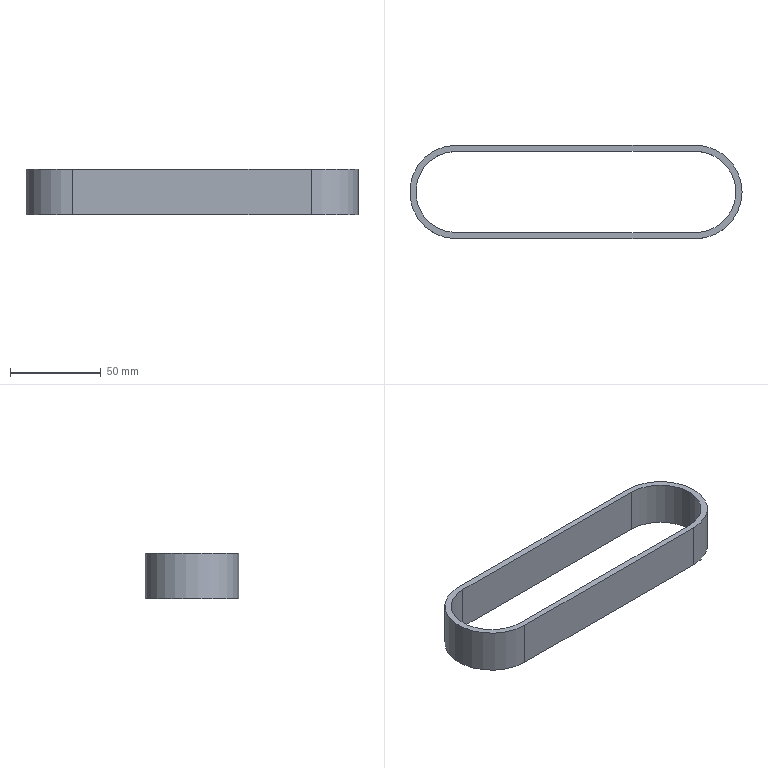Part | STEP file | 1 solid | 12 faces | box 183.34 x 51.65 x 25 mm | volume 35272 mm3 | cylinder 6 | plane 6 | commonest cylinder face diameters 44.85 x3 51.65 x3
STEP:
#1=CARTESIAN_POINT('',(0.,0.,0.));
#2=DIRECTION('',(0.,0.,1.));
#3=DIRECTION('',(1.,0.,0.));
#4=AXIS2_PLACEMENT_3D('',#1,#2,#3);
#5=CARTESIAN_POINT('',(8.226,1.112,-25.));
#6=VERTEX_POINT('',#5);
#7=CARTESIAN_POINT('',(8.226,1.112,0.));
#8=VERTEX_POINT('',#7);
#9=CARTESIAN_POINT('',(8.226,1.112,-25.));
#10=DIRECTION('',(0.,0.,1.));
#11=VECTOR('',#10,1.);
#12=LINE('',#9,#11);
#13=CARTESIAN_POINT('',(8.226,-21.313,-25.));
#14=DIRECTION('',(0.,0.,1.));
#15=DIRECTION('',(1.,0.,0.));
#16=AXIS2_PLACEMENT_3D('',#13,#14,#15);
#17=CYLINDRICAL_SURFACE('',#16,22.425);
#18=CARTESIAN_POINT('',(1.571,0.));
#19=DIRECTION('',(0.,1.));
#20=VECTOR('',#19,1.);
#21=LINE('',#18,#20);
#22=(GEOMETRIC_REPRESENTATION_CONTEXT(2)PARAMETRIC_REPRESENTATION_CONTEXT()REPRESENTATION_CONTEXT('',''));
#23=DEFINITIONAL_REPRESENTATION('',(#21),#22);
#24=PCURVE('',#17,#23);
#25=CARTESIAN_POINT('',(-123.465,1.112,-25.));
#26=DIRECTION('',(0.,-1.,0.));
#27=DIRECTION('',(0.,0.,-1.));
#28=AXIS2_PLACEMENT_3D('',#25,#26,#27);
#29=PLANE('',#28);
#30=CARTESIAN_POINT('',(0.,131.69));
#31=DIRECTION('',(-1.,0.));
#32=VECTOR('',#31,1.);
#33=LINE('',#30,#32);
#34=(GEOMETRIC_REPRESENTATION_CONTEXT(2)PARAMETRIC_REPRESENTATION_CONTEXT()REPRESENTATION_CONTEXT('',''));
#35=DEFINITIONAL_REPRESENTATION('',(#33),#34);
#36=PCURVE('',#29,#35);
#37=SURFACE_CURVE('',#12,(#24,#36),.PCURVE_S1.);
#38=EDGE_CURVE('',#6,#8,#37,.T.);
#39=ORIENTED_EDGE('',*,*,#38,.T.);
#40=CARTESIAN_POINT('',(30.651,-21.313,0.));
#41=VERTEX_POINT('',#40);
#42=CARTESIAN_POINT('',(8.226,-21.313,0.));
#43=DIRECTION('',(0.,0.,-1.));
#44=DIRECTION('',(-1.,0.,0.));
#45=AXIS2_PLACEMENT_3D('',#42,#43,#44);
#46=CIRCLE('',#45,22.425);
#47=CARTESIAN_POINT('',(3.142,25.));
#48=DIRECTION('',(-1.,0.));
#49=VECTOR('',#48,1.);
#50=LINE('',#47,#49);
#51=(GEOMETRIC_REPRESENTATION_CONTEXT(2)PARAMETRIC_REPRESENTATION_CONTEXT()REPRESENTATION_CONTEXT('',''));
#52=DEFINITIONAL_REPRESENTATION('',(#50),#51);
#53=PCURVE('',#17,#52);
#54=CARTESIAN_POINT('',(-123.465,-21.313,0.));
#55=DIRECTION('',(0.,0.,-1.));
#56=DIRECTION('',(-1.,0.,0.));
#57=AXIS2_PLACEMENT_3D('',#54,#55,#56);
#58=PLANE('',#57);
#59=CARTESIAN_POINT('',(-131.69,0.));
#60=DIRECTION('',(1.,0.));
#61=AXIS2_PLACEMENT_2D('',#59,#60);
#62=CIRCLE('',#61,22.425);
#63=(GEOMETRIC_REPRESENTATION_CONTEXT(2)PARAMETRIC_REPRESENTATION_CONTEXT()REPRESENTATION_CONTEXT('',''));
#64=DEFINITIONAL_REPRESENTATION('',(#62),#63);
#65=PCURVE('',#58,#64);
#66=SURFACE_CURVE('',#46,(#53,#65),.PCURVE_S1.);
#67=EDGE_CURVE('',#8,#41,#66,.T.);
#68=ORIENTED_EDGE('',*,*,#67,.T.);
#69=CARTESIAN_POINT('',(30.651,-21.313,-25.));
#70=VERTEX_POINT('',#69);
#71=CARTESIAN_POINT('',(30.651,-21.313,-25.));
#72=DIRECTION('',(0.,0.,1.));
#73=VECTOR('',#72,1.);
#74=LINE('',#71,#73);
#75=CARTESIAN_POINT('',(0.,0.));
#76=DIRECTION('',(0.,1.));
#77=VECTOR('',#76,1.);
#78=LINE('',#75,#77);
#79=(GEOMETRIC_REPRESENTATION_CONTEXT(2)PARAMETRIC_REPRESENTATION_CONTEXT()REPRESENTATION_CONTEXT('',''));
#80=DEFINITIONAL_REPRESENTATION('',(#78),#79);
#81=PCURVE('',#17,#80);
#82=CARTESIAN_POINT('',(8.226,-21.313,-25.));
#83=DIRECTION('',(0.,0.,1.));
#84=DIRECTION('',(1.,0.,0.));
#85=AXIS2_PLACEMENT_3D('',#82,#83,#84);
#86=CYLINDRICAL_SURFACE('',#85,22.425);
#87=CARTESIAN_POINT('',(6.283,0.));
#88=DIRECTION('',(0.,1.));
#89=VECTOR('',#88,1.);
#90=LINE('',#87,#89);
#91=(GEOMETRIC_REPRESENTATION_CONTEXT(2)PARAMETRIC_REPRESENTATION_CONTEXT()REPRESENTATION_CONTEXT('',''));
#92=DEFINITIONAL_REPRESENTATION('',(#90),#91);
#93=PCURVE('',#86,#92);
#94=SURFACE_CURVE('',#74,(#81,#93),.PCURVE_S1.);
#95=EDGE_CURVE('',#70,#41,#94,.T.);
#96=ORIENTED_EDGE('',*,*,#95,.F.);
#97=CARTESIAN_POINT('',(8.226,-21.313,-25.));
#98=DIRECTION('',(0.,0.,-1.));
#99=DIRECTION('',(-1.,0.,0.));
#100=AXIS2_PLACEMENT_3D('',#97,#98,#99);
#101=CIRCLE('',#100,22.425);
#102=CARTESIAN_POINT('',(3.142,0.));
#103=DIRECTION('',(-1.,0.));
#104=VECTOR('',#103,1.);
#105=LINE('',#102,#104);
#106=(GEOMETRIC_REPRESENTATION_CONTEXT(2)PARAMETRIC_REPRESENTATION_CONTEXT()REPRESENTATION_CONTEXT('',''));
#107=DEFINITIONAL_REPRESENTATION('',(#105),#106);
#108=PCURVE('',#17,#107);
#109=CARTESIAN_POINT('',(-123.465,-21.313,-25.));
#110=DIRECTION('',(0.,0.,-1.));
#111=DIRECTION('',(-1.,0.,0.));
#112=AXIS2_PLACEMENT_3D('',#109,#110,#111);
#113=PLANE('',#112);
#114=CARTESIAN_POINT('',(-131.69,0.));
#115=DIRECTION('',(1.,0.));
#116=AXIS2_PLACEMENT_2D('',#114,#115);
#117=CIRCLE('',#116,22.425);
#118=(GEOMETRIC_REPRESENTATION_CONTEXT(2)PARAMETRIC_REPRESENTATION_CONTEXT()REPRESENTATION_CONTEXT('',''));
#119=DEFINITIONAL_REPRESENTATION('',(#117),#118);
#120=PCURVE('',#113,#119);
#121=SURFACE_CURVE('',#101,(#108,#120),.PCURVE_S1.);
#122=EDGE_CURVE('',#6,#70,#121,.T.);
#123=ORIENTED_EDGE('',*,*,#122,.F.);
#124=EDGE_LOOP('',(#39,#68,#96,#123));
#125=FACE_BOUND('',#124,.F.);
#126=ADVANCED_FACE('',(#125),#17,.F.);
#127=CARTESIAN_POINT('',(34.051,-21.313,-25.));
#128=VERTEX_POINT('',#127);
#129=CARTESIAN_POINT('',(8.226,-47.138,-25.));
#130=VERTEX_POINT('',#129);
#131=CARTESIAN_POINT('',(8.226,-21.313,-25.));
#132=DIRECTION('',(0.,0.,-1.));
#133=DIRECTION('',(-1.,0.,0.));
#134=AXIS2_PLACEMENT_3D('',#131,#132,#133);
#135=CIRCLE('',#134,25.825);
#136=CARTESIAN_POINT('',(8.226,-21.313,-25.));
#137=DIRECTION('',(0.,0.,1.));
#138=DIRECTION('',(1.,0.,0.));
#139=AXIS2_PLACEMENT_3D('',#136,#137,#138);
#140=CYLINDRICAL_SURFACE('',#139,25.825);
#141=CARTESIAN_POINT('',(9.425,0.));
#142=DIRECTION('',(-1.,0.));
#143=VECTOR('',#142,1.);
#144=LINE('',#141,#143);
#145=(GEOMETRIC_REPRESENTATION_CONTEXT(2)PARAMETRIC_REPRESENTATION_CONTEXT()REPRESENTATION_CONTEXT('',''));
#146=DEFINITIONAL_REPRESENTATION('',(#144),#145);
#147=PCURVE('',#140,#146);
#148=CARTESIAN_POINT('',(-131.69,0.));
#149=DIRECTION('',(1.,0.));
#150=AXIS2_PLACEMENT_2D('',#148,#149);
#151=CIRCLE('',#150,25.825);
#152=(GEOMETRIC_REPRESENTATION_CONTEXT(2)PARAMETRIC_REPRESENTATION_CONTEXT()REPRESENTATION_CONTEXT('',''));
#153=DEFINITIONAL_REPRESENTATION('',(#151),#152);
#154=PCURVE('',#113,#153);
#155=SURFACE_CURVE('',#135,(#147,#154),.PCURVE_S1.);
#156=EDGE_CURVE('',#128,#130,#155,.T.);
#157=ORIENTED_EDGE('',*,*,#156,.F.);
#158=CARTESIAN_POINT('',(34.051,-21.313,0.));
#159=VERTEX_POINT('',#158);
#160=CARTESIAN_POINT('',(34.051,-21.313,-25.));
#161=DIRECTION('',(0.,0.,1.));
#162=VECTOR('',#161,1.);
#163=LINE('',#160,#162);
#164=CARTESIAN_POINT('',(6.283,0.));
#165=DIRECTION('',(0.,1.));
#166=VECTOR('',#165,1.);
#167=LINE('',#164,#166);
#168=(GEOMETRIC_REPRESENTATION_CONTEXT(2)PARAMETRIC_REPRESENTATION_CONTEXT()REPRESENTATION_CONTEXT('',''));
#169=DEFINITIONAL_REPRESENTATION('',(#167),#168);
#170=PCURVE('',#140,#169);
#171=CARTESIAN_POINT('',(8.226,-21.313,-25.));
#172=DIRECTION('',(0.,0.,1.));
#173=DIRECTION('',(1.,0.,0.));
#174=AXIS2_PLACEMENT_3D('',#171,#172,#173);
#175=CYLINDRICAL_SURFACE('',#174,25.825);
#176=CARTESIAN_POINT('',(0.,0.));
#177=DIRECTION('',(0.,1.));
#178=VECTOR('',#177,1.);
#179=LINE('',#176,#178);
#180=(GEOMETRIC_REPRESENTATION_CONTEXT(2)PARAMETRIC_REPRESENTATION_CONTEXT()REPRESENTATION_CONTEXT('',''));
#181=DEFINITIONAL_REPRESENTATION('',(#179),#180);
#182=PCURVE('',#175,#181);
#183=SURFACE_CURVE('',#163,(#170,#182),.PCURVE_S1.);
#184=EDGE_CURVE('',#128,#159,#183,.T.);
#185=ORIENTED_EDGE('',*,*,#184,.T.);
#186=CARTESIAN_POINT('',(8.226,-47.138,0.));
#187=VERTEX_POINT('',#186);
#188=CARTESIAN_POINT('',(8.226,-21.313,0.));
#189=DIRECTION('',(0.,0.,-1.));
#190=DIRECTION('',(-1.,0.,0.));
#191=AXIS2_PLACEMENT_3D('',#188,#189,#190);
#192=CIRCLE('',#191,25.825);
#193=CARTESIAN_POINT('',(9.425,25.));
#194=DIRECTION('',(-1.,0.));
#195=VECTOR('',#194,1.);
#196=LINE('',#193,#195);
#197=(GEOMETRIC_REPRESENTATION_CONTEXT(2)PARAMETRIC_REPRESENTATION_CONTEXT()REPRESENTATION_CONTEXT('',''));
#198=DEFINITIONAL_REPRESENTATION('',(#196),#197);
#199=PCURVE('',#140,#198);
#200=CARTESIAN_POINT('',(-131.69,0.));
#201=DIRECTION('',(1.,0.));
#202=AXIS2_PLACEMENT_2D('',#200,#201);
#203=CIRCLE('',#202,25.825);
#204=(GEOMETRIC_REPRESENTATION_CONTEXT(2)PARAMETRIC_REPRESENTATION_CONTEXT()REPRESENTATION_CONTEXT('',''));
#205=DEFINITIONAL_REPRESENTATION('',(#203),#204);
#206=PCURVE('',#58,#205);
#207=SURFACE_CURVE('',#192,(#199,#206),.PCURVE_S1.);
#208=EDGE_CURVE('',#159,#187,#207,.T.);
#209=ORIENTED_EDGE('',*,*,#208,.T.);
#210=CARTESIAN_POINT('',(8.226,-47.138,-25.));
#211=DIRECTION('',(0.,0.,1.));
#212=VECTOR('',#211,1.);
#213=LINE('',#210,#212);
#214=CARTESIAN_POINT('',(4.712,0.));
#215=DIRECTION('',(0.,1.));
#216=VECTOR('',#215,1.);
#217=LINE('',#214,#216);
#218=(GEOMETRIC_REPRESENTATION_CONTEXT(2)PARAMETRIC_REPRESENTATION_CONTEXT()REPRESENTATION_CONTEXT('',''));
#219=DEFINITIONAL_REPRESENTATION('',(#217),#218);
#220=PCURVE('',#140,#219);
#221=CARTESIAN_POINT('',(-123.465,-47.138,-25.));
#222=DIRECTION('',(0.,1.,0.));
#223=DIRECTION('',(0.,0.,1.));
#224=AXIS2_PLACEMENT_3D('',#221,#222,#223);
#225=PLANE('',#224);
#226=CARTESIAN_POINT('',(0.,131.69));
#227=DIRECTION('',(1.,0.));
#228=VECTOR('',#227,1.);
#229=LINE('',#226,#228);
#230=(GEOMETRIC_REPRESENTATION_CONTEXT(2)PARAMETRIC_REPRESENTATION_CONTEXT()REPRESENTATION_CONTEXT('',''));
#231=DEFINITIONAL_REPRESENTATION('',(#229),#230);
#232=PCURVE('',#225,#231);
#233=SURFACE_CURVE('',#213,(#220,#232),.PCURVE_S1.);
#234=EDGE_CURVE('',#130,#187,#233,.T.);
#235=ORIENTED_EDGE('',*,*,#234,.F.);
#236=EDGE_LOOP('',(#157,#185,#209,#235));
#237=FACE_BOUND('',#236,.T.);
#238=ADVANCED_FACE('',(#237),#140,.T.);
#239=CARTESIAN_POINT('',(-123.465,-47.138,-25.));
#240=VERTEX_POINT('',#239);
#241=CARTESIAN_POINT('',(-123.465,4.512,-25.));
#242=VERTEX_POINT('',#241);
#243=CARTESIAN_POINT('',(-123.465,-21.313,-25.));
#244=DIRECTION('',(0.,0.,-1.));
#245=DIRECTION('',(-1.,0.,0.));
#246=AXIS2_PLACEMENT_3D('',#243,#244,#245);
#247=CIRCLE('',#246,25.825);
#248=CARTESIAN_POINT('',(0.,0.));
#249=DIRECTION('',(1.,0.));
#250=AXIS2_PLACEMENT_2D('',#248,#249);
#251=CIRCLE('',#250,25.825);
#252=(GEOMETRIC_REPRESENTATION_CONTEXT(2)PARAMETRIC_REPRESENTATION_CONTEXT()REPRESENTATION_CONTEXT('',''));
#253=DEFINITIONAL_REPRESENTATION('',(#251),#252);
#254=PCURVE('',#113,#253);
#255=CARTESIAN_POINT('',(-123.465,-21.313,-25.));
#256=DIRECTION('',(0.,0.,1.));
#257=DIRECTION('',(1.,0.,0.));
#258=AXIS2_PLACEMENT_3D('',#255,#256,#257);
#259=CYLINDRICAL_SURFACE('',#258,25.825);
#260=CARTESIAN_POINT('',(9.425,0.));
#261=DIRECTION('',(-1.,0.));
#262=VECTOR('',#261,1.);
#263=LINE('',#260,#262);
#264=(GEOMETRIC_REPRESENTATION_CONTEXT(2)PARAMETRIC_REPRESENTATION_CONTEXT()REPRESENTATION_CONTEXT('',''));
#265=DEFINITIONAL_REPRESENTATION('',(#263),#264);
#266=PCURVE('',#259,#265);
#267=SURFACE_CURVE('',#247,(#254,#266),.PCURVE_S1.);
#268=EDGE_CURVE('',#240,#242,#267,.T.);
#269=ORIENTED_EDGE('',*,*,#268,.T.);
#270=CARTESIAN_POINT('',(8.226,4.512,-25.));
#271=VERTEX_POINT('',#270);
#272=CARTESIAN_POINT('',(-123.465,4.512,-25.));
#273=DIRECTION('',(1.,0.,0.));
#274=VECTOR('',#273,1.);
#275=LINE('',#272,#274);
#276=CARTESIAN_POINT('',(0.,25.825));
#277=DIRECTION('',(-1.,0.));
#278=VECTOR('',#277,1.);
#279=LINE('',#276,#278);
#280=(GEOMETRIC_REPRESENTATION_CONTEXT(2)PARAMETRIC_REPRESENTATION_CONTEXT()REPRESENTATION_CONTEXT('',''));
#281=DEFINITIONAL_REPRESENTATION('',(#279),#280);
#282=PCURVE('',#113,#281);
#283=CARTESIAN_POINT('',(-123.465,4.512,-25.));
#284=DIRECTION('',(0.,-1.,0.));
#285=DIRECTION('',(0.,0.,-1.));
#286=AXIS2_PLACEMENT_3D('',#283,#284,#285);
#287=PLANE('',#286);
#288=CARTESIAN_POINT('',(0.,0.));
#289=DIRECTION('',(0.,1.));
#290=VECTOR('',#289,1.);
#291=LINE('',#288,#290);
#292=(GEOMETRIC_REPRESENTATION_CONTEXT(2)PARAMETRIC_REPRESENTATION_CONTEXT()REPRESENTATION_CONTEXT('',''));
#293=DEFINITIONAL_REPRESENTATION('',(#291),#292);
#294=PCURVE('',#287,#293);
#295=SURFACE_CURVE('',#275,(#282,#294),.PCURVE_S1.);
#296=EDGE_CURVE('',#242,#271,#295,.T.);
#297=ORIENTED_EDGE('',*,*,#296,.T.);
#298=CARTESIAN_POINT('',(8.226,-21.313,-25.));
#299=DIRECTION('',(0.,0.,-1.));
#300=DIRECTION('',(-1.,0.,0.));
#301=AXIS2_PLACEMENT_3D('',#298,#299,#300);
#302=CIRCLE('',#301,25.825);
#303=CARTESIAN_POINT('',(-131.69,0.));
#304=DIRECTION('',(1.,0.));
#305=AXIS2_PLACEMENT_2D('',#303,#304);
#306=CIRCLE('',#305,25.825);
#307=(GEOMETRIC_REPRESENTATION_CONTEXT(2)PARAMETRIC_REPRESENTATION_CONTEXT()REPRESENTATION_CONTEXT('',''));
#308=DEFINITIONAL_REPRESENTATION('',(#306),#307);
#309=PCURVE('',#113,#308);
#310=CARTESIAN_POINT('',(3.142,0.));
#311=DIRECTION('',(-1.,0.));
#312=VECTOR('',#311,1.);
#313=LINE('',#310,#312);
#314=(GEOMETRIC_REPRESENTATION_CONTEXT(2)PARAMETRIC_REPRESENTATION_CONTEXT()REPRESENTATION_CONTEXT('',''));
#315=DEFINITIONAL_REPRESENTATION('',(#313),#314);
#316=PCURVE('',#175,#315);
#317=SURFACE_CURVE('',#302,(#309,#316),.PCURVE_S1.);
#318=EDGE_CURVE('',#271,#128,#317,.T.);
#319=ORIENTED_EDGE('',*,*,#318,.T.);
#320=ORIENTED_EDGE('',*,*,#156,.T.);
#321=CARTESIAN_POINT('',(-123.465,-47.138,-25.));
#322=DIRECTION('',(-1.,0.,0.));
#323=VECTOR('',#322,1.);
#324=LINE('',#321,#323);
#325=CARTESIAN_POINT('',(0.,-25.825));
#326=DIRECTION('',(1.,0.));
#327=VECTOR('',#326,1.);
#328=LINE('',#325,#327);
#329=(GEOMETRIC_REPRESENTATION_CONTEXT(2)PARAMETRIC_REPRESENTATION_CONTEXT()REPRESENTATION_CONTEXT('',''));
#330=DEFINITIONAL_REPRESENTATION('',(#328),#329);
#331=PCURVE('',#113,#330);
#332=CARTESIAN_POINT('',(0.,0.));
#333=DIRECTION('',(0.,-1.));
#334=VECTOR('',#333,1.);
#335=LINE('',#332,#334);
#336=(GEOMETRIC_REPRESENTATION_CONTEXT(2)PARAMETRIC_REPRESENTATION_CONTEXT()REPRESENTATION_CONTEXT('',''));
#337=DEFINITIONAL_REPRESENTATION('',(#335),#336);
#338=PCURVE('',#225,#337);
#339=SURFACE_CURVE('',#324,(#331,#338),.PCURVE_S1.);
#340=EDGE_CURVE('',#130,#240,#339,.T.);
#341=ORIENTED_EDGE('',*,*,#340,.T.);
#342=EDGE_LOOP('',(#269,#297,#319,#320,#341));
#343=FACE_BOUND('',#342,.T.);
#344=CARTESIAN_POINT('',(-123.465,1.112,-25.));
#345=VERTEX_POINT('',#344);
#346=CARTESIAN_POINT('',(-123.465,1.112,-25.));
#347=DIRECTION('',(1.,0.,0.));
#348=VECTOR('',#347,1.);
#349=LINE('',#346,#348);
#350=CARTESIAN_POINT('',(0.,22.425));
#351=DIRECTION('',(-1.,0.));
#352=VECTOR('',#351,1.);
#353=LINE('',#350,#352);
#354=(GEOMETRIC_REPRESENTATION_CONTEXT(2)PARAMETRIC_REPRESENTATION_CONTEXT()REPRESENTATION_CONTEXT('',''));
#355=DEFINITIONAL_REPRESENTATION('',(#353),#354);
#356=PCURVE('',#113,#355);
#357=CARTESIAN_POINT('',(0.,0.));
#358=DIRECTION('',(0.,1.));
#359=VECTOR('',#358,1.);
#360=LINE('',#357,#359);
#361=(GEOMETRIC_REPRESENTATION_CONTEXT(2)PARAMETRIC_REPRESENTATION_CONTEXT()REPRESENTATION_CONTEXT('',''));
#362=DEFINITIONAL_REPRESENTATION('',(#360),#361);
#363=PCURVE('',#29,#362);
#364=SURFACE_CURVE('',#349,(#356,#363),.PCURVE_S1.);
#365=EDGE_CURVE('',#345,#6,#364,.T.);
#366=ORIENTED_EDGE('',*,*,#365,.F.);
#367=CARTESIAN_POINT('',(-123.465,-43.738,-25.));
#368=VERTEX_POINT('',#367);
#369=CARTESIAN_POINT('',(-123.465,-21.313,-25.));
#370=DIRECTION('',(0.,0.,-1.));
#371=DIRECTION('',(-1.,0.,0.));
#372=AXIS2_PLACEMENT_3D('',#369,#370,#371);
#373=CIRCLE('',#372,22.425);
#374=CARTESIAN_POINT('',(0.,0.));
#375=DIRECTION('',(1.,0.));
#376=AXIS2_PLACEMENT_2D('',#374,#375);
#377=CIRCLE('',#376,22.425);
#378=(GEOMETRIC_REPRESENTATION_CONTEXT(2)PARAMETRIC_REPRESENTATION_CONTEXT()REPRESENTATION_CONTEXT('',''));
#379=DEFINITIONAL_REPRESENTATION('',(#377),#378);
#380=PCURVE('',#113,#379);
#381=CARTESIAN_POINT('',(-123.465,-21.313,-25.));
#382=DIRECTION('',(0.,0.,1.));
#383=DIRECTION('',(1.,0.,0.));
#384=AXIS2_PLACEMENT_3D('',#381,#382,#383);
#385=CYLINDRICAL_SURFACE('',#384,22.425);
#386=CARTESIAN_POINT('',(9.425,0.));
#387=DIRECTION('',(-1.,0.));
#388=VECTOR('',#387,1.);
#389=LINE('',#386,#388);
#390=(GEOMETRIC_REPRESENTATION_CONTEXT(2)PARAMETRIC_REPRESENTATION_CONTEXT()REPRESENTATION_CONTEXT('',''));
#391=DEFINITIONAL_REPRESENTATION('',(#389),#390);
#392=PCURVE('',#385,#391);
#393=SURFACE_CURVE('',#373,(#380,#392),.PCURVE_S1.);
#394=EDGE_CURVE('',#368,#345,#393,.T.);
#395=ORIENTED_EDGE('',*,*,#394,.F.);
#396=CARTESIAN_POINT('',(8.226,-43.738,-25.));
#397=VERTEX_POINT('',#396);
#398=CARTESIAN_POINT('',(-123.465,-43.738,-25.));
#399=DIRECTION('',(-1.,0.,0.));
#400=VECTOR('',#399,1.);
#401=LINE('',#398,#400);
#402=CARTESIAN_POINT('',(0.,-22.425));
#403=DIRECTION('',(1.,0.));
#404=VECTOR('',#403,1.);
#405=LINE('',#402,#404);
#406=(GEOMETRIC_REPRESENTATION_CONTEXT(2)PARAMETRIC_REPRESENTATION_CONTEXT()REPRESENTATION_CONTEXT('',''));
#407=DEFINITIONAL_REPRESENTATION('',(#405),#406);
#408=PCURVE('',#113,#407);
#409=CARTESIAN_POINT('',(-123.465,-43.738,-25.));
#410=DIRECTION('',(0.,1.,0.));
#411=DIRECTION('',(0.,0.,1.));
#412=AXIS2_PLACEMENT_3D('',#409,#410,#411);
#413=PLANE('',#412);
#414=CARTESIAN_POINT('',(0.,0.));
#415=DIRECTION('',(0.,-1.));
#416=VECTOR('',#415,1.);
#417=LINE('',#414,#416);
#418=(GEOMETRIC_REPRESENTATION_CONTEXT(2)PARAMETRIC_REPRESENTATION_CONTEXT()REPRESENTATION_CONTEXT('',''));
#419=DEFINITIONAL_REPRESENTATION('',(#417),#418);
#420=PCURVE('',#413,#419);
#421=SURFACE_CURVE('',#401,(#408,#420),.PCURVE_S1.);
#422=EDGE_CURVE('',#397,#368,#421,.T.);
#423=ORIENTED_EDGE('',*,*,#422,.F.);
#424=CARTESIAN_POINT('',(8.226,-21.313,-25.));
#425=DIRECTION('',(0.,0.,-1.));
#426=DIRECTION('',(-1.,0.,0.));
#427=AXIS2_PLACEMENT_3D('',#424,#425,#426);
#428=CIRCLE('',#427,22.425);
#429=CARTESIAN_POINT('',(-131.69,0.));
#430=DIRECTION('',(1.,0.));
#431=AXIS2_PLACEMENT_2D('',#429,#430);
#432=CIRCLE('',#431,22.425);
#433=(GEOMETRIC_REPRESENTATION_CONTEXT(2)PARAMETRIC_REPRESENTATION_CONTEXT()REPRESENTATION_CONTEXT('',''));
#434=DEFINITIONAL_REPRESENTATION('',(#432),#433);
#435=PCURVE('',#113,#434);
#436=CARTESIAN_POINT('',(9.425,0.));
#437=DIRECTION('',(-1.,0.));
#438=VECTOR('',#437,1.);
#439=LINE('',#436,#438);
#440=(GEOMETRIC_REPRESENTATION_CONTEXT(2)PARAMETRIC_REPRESENTATION_CONTEXT()REPRESENTATION_CONTEXT('',''));
#441=DEFINITIONAL_REPRESENTATION('',(#439),#440);
#442=PCURVE('',#86,#441);
#443=SURFACE_CURVE('',#428,(#435,#442),.PCURVE_S1.);
#444=EDGE_CURVE('',#70,#397,#443,.T.);
#445=ORIENTED_EDGE('',*,*,#444,.F.);
#446=ORIENTED_EDGE('',*,*,#122,.F.);
#447=EDGE_LOOP('',(#366,#395,#423,#445,#446));
#448=FACE_BOUND('',#447,.T.);
#449=ADVANCED_FACE('',(#343,#448),#113,.T.);
#450=CARTESIAN_POINT('',(-123.465,-47.138,0.));
#451=VERTEX_POINT('',#450);
#452=CARTESIAN_POINT('',(-123.465,4.512,0.));
#453=VERTEX_POINT('',#452);
#454=CARTESIAN_POINT('',(-123.465,-21.313,0.));
#455=DIRECTION('',(0.,0.,-1.));
#456=DIRECTION('',(-1.,0.,0.));
#457=AXIS2_PLACEMENT_3D('',#454,#455,#456);
#458=CIRCLE('',#457,25.825);
#459=CARTESIAN_POINT('',(0.,0.));
#460=DIRECTION('',(1.,0.));
#461=AXIS2_PLACEMENT_2D('',#459,#460);
#462=CIRCLE('',#461,25.825);
#463=(GEOMETRIC_REPRESENTATION_CONTEXT(2)PARAMETRIC_REPRESENTATION_CONTEXT()REPRESENTATION_CONTEXT('',''));
#464=DEFINITIONAL_REPRESENTATION('',(#462),#463);
#465=PCURVE('',#58,#464);
#466=CARTESIAN_POINT('',(9.425,25.));
#467=DIRECTION('',(-1.,0.));
#468=VECTOR('',#467,1.);
#469=LINE('',#466,#468);
#470=(GEOMETRIC_REPRESENTATION_CONTEXT(2)PARAMETRIC_REPRESENTATION_CONTEXT()REPRESENTATION_CONTEXT('',''));
#471=DEFINITIONAL_REPRESENTATION('',(#469),#470);
#472=PCURVE('',#259,#471);
#473=SURFACE_CURVE('',#458,(#465,#472),.PCURVE_S1.);
#474=EDGE_CURVE('',#451,#453,#473,.T.);
#475=ORIENTED_EDGE('',*,*,#474,.F.);
#476=CARTESIAN_POINT('',(-123.465,-47.138,0.));
#477=DIRECTION('',(-1.,0.,0.));
#478=VECTOR('',#477,1.);
#479=LINE('',#476,#478);
#480=CARTESIAN_POINT('',(0.,-25.825));
#481=DIRECTION('',(1.,0.));
#482=VECTOR('',#481,1.);
#483=LINE('',#480,#482);
#484=(GEOMETRIC_REPRESENTATION_CONTEXT(2)PARAMETRIC_REPRESENTATION_CONTEXT()REPRESENTATION_CONTEXT('',''));
#485=DEFINITIONAL_REPRESENTATION('',(#483),#484);
#486=PCURVE('',#58,#485);
#487=CARTESIAN_POINT('',(25.,0.));
#488=DIRECTION('',(0.,-1.));
#489=VECTOR('',#488,1.);
#490=LINE('',#487,#489);
#491=(GEOMETRIC_REPRESENTATION_CONTEXT(2)PARAMETRIC_REPRESENTATION_CONTEXT()REPRESENTATION_CONTEXT('',''));
#492=DEFINITIONAL_REPRESENTATION('',(#490),#491);
#493=PCURVE('',#225,#492);
#494=SURFACE_CURVE('',#479,(#486,#493),.PCURVE_S1.);
#495=EDGE_CURVE('',#187,#451,#494,.T.);
#496=ORIENTED_EDGE('',*,*,#495,.F.);
#497=ORIENTED_EDGE('',*,*,#208,.F.);
#498=CARTESIAN_POINT('',(8.226,4.512,0.));
#499=VERTEX_POINT('',#498);
#500=CARTESIAN_POINT('',(8.226,-21.313,0.));
#501=DIRECTION('',(0.,0.,-1.));
#502=DIRECTION('',(-1.,0.,0.));
#503=AXIS2_PLACEMENT_3D('',#500,#501,#502);
#504=CIRCLE('',#503,25.825);
#505=CARTESIAN_POINT('',(-131.69,0.));
#506=DIRECTION('',(1.,0.));
#507=AXIS2_PLACEMENT_2D('',#505,#506);
#508=CIRCLE('',#507,25.825);
#509=(GEOMETRIC_REPRESENTATION_CONTEXT(2)PARAMETRIC_REPRESENTATION_CONTEXT()REPRESENTATION_CONTEXT('',''));
#510=DEFINITIONAL_REPRESENTATION('',(#508),#509);
#511=PCURVE('',#58,#510);
#512=CARTESIAN_POINT('',(3.142,25.));
#513=DIRECTION('',(-1.,0.));
#514=VECTOR('',#513,1.);
#515=LINE('',#512,#514);
#516=(GEOMETRIC_REPRESENTATION_CONTEXT(2)PARAMETRIC_REPRESENTATION_CONTEXT()REPRESENTATION_CONTEXT('',''));
#517=DEFINITIONAL_REPRESENTATION('',(#515),#516);
#518=PCURVE('',#175,#517);
#519=SURFACE_CURVE('',#504,(#511,#518),.PCURVE_S1.);
#520=EDGE_CURVE('',#499,#159,#519,.T.);
#521=ORIENTED_EDGE('',*,*,#520,.F.);
#522=CARTESIAN_POINT('',(-123.465,4.512,0.));
#523=DIRECTION('',(1.,0.,0.));
#524=VECTOR('',#523,1.);
#525=LINE('',#522,#524);
#526=CARTESIAN_POINT('',(0.,25.825));
#527=DIRECTION('',(-1.,0.));
#528=VECTOR('',#527,1.);
#529=LINE('',#526,#528);
#530=(GEOMETRIC_REPRESENTATION_CONTEXT(2)PARAMETRIC_REPRESENTATION_CONTEXT()REPRESENTATION_CONTEXT('',''));
#531=DEFINITIONAL_REPRESENTATION('',(#529),#530);
#532=PCURVE('',#58,#531);
#533=CARTESIAN_POINT('',(-25.,0.));
#534=DIRECTION('',(0.,1.));
#535=VECTOR('',#534,1.);
#536=LINE('',#533,#535);
#537=(GEOMETRIC_REPRESENTATION_CONTEXT(2)PARAMETRIC_REPRESENTATION_CONTEXT()REPRESENTATION_CONTEXT('',''));
#538=DEFINITIONAL_REPRESENTATION('',(#536),#537);
#539=PCURVE('',#287,#538);
#540=SURFACE_CURVE('',#525,(#532,#539),.PCURVE_S1.);
#541=EDGE_CURVE('',#453,#499,#540,.T.);
#542=ORIENTED_EDGE('',*,*,#541,.F.);
#543=EDGE_LOOP('',(#475,#496,#497,#521,#542));
#544=FACE_BOUND('',#543,.T.);
#545=CARTESIAN_POINT('',(-123.465,-43.738,0.));
#546=VERTEX_POINT('',#545);
#547=CARTESIAN_POINT('',(-123.465,1.112,0.));
#548=VERTEX_POINT('',#547);
#549=CARTESIAN_POINT('',(-123.465,-21.313,0.));
#550=DIRECTION('',(0.,0.,-1.));
#551=DIRECTION('',(-1.,0.,0.));
#552=AXIS2_PLACEMENT_3D('',#549,#550,#551);
#553=CIRCLE('',#552,22.425);
#554=CARTESIAN_POINT('',(0.,0.));
#555=DIRECTION('',(1.,0.));
#556=AXIS2_PLACEMENT_2D('',#554,#555);
#557=CIRCLE('',#556,22.425);
#558=(GEOMETRIC_REPRESENTATION_CONTEXT(2)PARAMETRIC_REPRESENTATION_CONTEXT()REPRESENTATION_CONTEXT('',''));
#559=DEFINITIONAL_REPRESENTATION('',(#557),#558);
#560=PCURVE('',#58,#559);
#561=CARTESIAN_POINT('',(9.425,25.));
#562=DIRECTION('',(-1.,0.));
#563=VECTOR('',#562,1.);
#564=LINE('',#561,#563);
#565=(GEOMETRIC_REPRESENTATION_CONTEXT(2)PARAMETRIC_REPRESENTATION_CONTEXT()REPRESENTATION_CONTEXT('',''));
#566=DEFINITIONAL_REPRESENTATION('',(#564),#565);
#567=PCURVE('',#385,#566);
#568=SURFACE_CURVE('',#553,(#560,#567),.PCURVE_S1.);
#569=EDGE_CURVE('',#546,#548,#568,.T.);
#570=ORIENTED_EDGE('',*,*,#569,.T.);
#571=CARTESIAN_POINT('',(-123.465,1.112,0.));
#572=DIRECTION('',(1.,0.,0.));
#573=VECTOR('',#572,1.);
#574=LINE('',#571,#573);
#575=CARTESIAN_POINT('',(0.,22.425));
#576=DIRECTION('',(-1.,0.));
#577=VECTOR('',#576,1.);
#578=LINE('',#575,#577);
#579=(GEOMETRIC_REPRESENTATION_CONTEXT(2)PARAMETRIC_REPRESENTATION_CONTEXT()REPRESENTATION_CONTEXT('',''));
#580=DEFINITIONAL_REPRESENTATION('',(#578),#579);
#581=PCURVE('',#58,#580);
#582=CARTESIAN_POINT('',(-25.,0.));
#583=DIRECTION('',(0.,1.));
#584=VECTOR('',#583,1.);
#585=LINE('',#582,#584);
#586=(GEOMETRIC_REPRESENTATION_CONTEXT(2)PARAMETRIC_REPRESENTATION_CONTEXT()REPRESENTATION_CONTEXT('',''));
#587=DEFINITIONAL_REPRESENTATION('',(#585),#586);
#588=PCURVE('',#29,#587);
#589=SURFACE_CURVE('',#574,(#581,#588),.PCURVE_S1.);
#590=EDGE_CURVE('',#548,#8,#589,.T.);
#591=ORIENTED_EDGE('',*,*,#590,.T.);
#592=ORIENTED_EDGE('',*,*,#67,.T.);
#593=CARTESIAN_POINT('',(8.226,-43.738,0.));
#594=VERTEX_POINT('',#593);
#595=CARTESIAN_POINT('',(8.226,-21.313,0.));
#596=DIRECTION('',(0.,0.,-1.));
#597=DIRECTION('',(-1.,0.,0.));
#598=AXIS2_PLACEMENT_3D('',#595,#596,#597);
#599=CIRCLE('',#598,22.425);
#600=CARTESIAN_POINT('',(-131.69,0.));
#601=DIRECTION('',(1.,0.));
#602=AXIS2_PLACEMENT_2D('',#600,#601);
#603=CIRCLE('',#602,22.425);
#604=(GEOMETRIC_REPRESENTATION_CONTEXT(2)PARAMETRIC_REPRESENTATION_CONTEXT()REPRESENTATION_CONTEXT('',''));
#605=DEFINITIONAL_REPRESENTATION('',(#603),#604);
#606=PCURVE('',#58,#605);
#607=CARTESIAN_POINT('',(9.425,25.));
#608=DIRECTION('',(-1.,0.));
#609=VECTOR('',#608,1.);
#610=LINE('',#607,#609);
#611=(GEOMETRIC_REPRESENTATION_CONTEXT(2)PARAMETRIC_REPRESENTATION_CONTEXT()REPRESENTATION_CONTEXT('',''));
#612=DEFINITIONAL_REPRESENTATION('',(#610),#611);
#613=PCURVE('',#86,#612);
#614=SURFACE_CURVE('',#599,(#606,#613),.PCURVE_S1.);
#615=EDGE_CURVE('',#41,#594,#614,.T.);
#616=ORIENTED_EDGE('',*,*,#615,.T.);
#617=CARTESIAN_POINT('',(-123.465,-43.738,0.));
#618=DIRECTION('',(-1.,0.,0.));
#619=VECTOR('',#618,1.);
#620=LINE('',#617,#619);
#621=CARTESIAN_POINT('',(0.,-22.425));
#622=DIRECTION('',(1.,0.));
#623=VECTOR('',#622,1.);
#624=LINE('',#621,#623);
#625=(GEOMETRIC_REPRESENTATION_CONTEXT(2)PARAMETRIC_REPRESENTATION_CONTEXT()REPRESENTATION_CONTEXT('',''));
#626=DEFINITIONAL_REPRESENTATION('',(#624),#625);
#627=PCURVE('',#58,#626);
#628=CARTESIAN_POINT('',(25.,0.));
#629=DIRECTION('',(0.,-1.));
#630=VECTOR('',#629,1.);
#631=LINE('',#628,#630);
#632=(GEOMETRIC_REPRESENTATION_CONTEXT(2)PARAMETRIC_REPRESENTATION_CONTEXT()REPRESENTATION_CONTEXT('',''));
#633=DEFINITIONAL_REPRESENTATION('',(#631),#632);
#634=PCURVE('',#413,#633);
#635=SURFACE_CURVE('',#620,(#627,#634),.PCURVE_S1.);
#636=EDGE_CURVE('',#594,#546,#635,.T.);
#637=ORIENTED_EDGE('',*,*,#636,.T.);
#638=EDGE_LOOP('',(#570,#591,#592,#616,#637));
#639=FACE_BOUND('',#638,.T.);
#640=ADVANCED_FACE('',(#544,#639),#58,.F.);
#641=ORIENTED_EDGE('',*,*,#474,.T.);
#642=CARTESIAN_POINT('',(-123.465,4.512,-25.));
#643=DIRECTION('',(0.,0.,1.));
#644=VECTOR('',#643,1.);
#645=LINE('',#642,#644);
#646=CARTESIAN_POINT('',(1.571,0.));
#647=DIRECTION('',(0.,1.));
#648=VECTOR('',#647,1.);
#649=LINE('',#646,#648);
#650=(GEOMETRIC_REPRESENTATION_CONTEXT(2)PARAMETRIC_REPRESENTATION_CONTEXT()REPRESENTATION_CONTEXT('',''));
#651=DEFINITIONAL_REPRESENTATION('',(#649),#650);
#652=PCURVE('',#259,#651);
#653=CARTESIAN_POINT('',(0.,0.));
#654=DIRECTION('',(-1.,0.));
#655=VECTOR('',#654,1.);
#656=LINE('',#653,#655);
#657=(GEOMETRIC_REPRESENTATION_CONTEXT(2)PARAMETRIC_REPRESENTATION_CONTEXT()REPRESENTATION_CONTEXT('',''));
#658=DEFINITIONAL_REPRESENTATION('',(#656),#657);
#659=PCURVE('',#287,#658);
#660=SURFACE_CURVE('',#645,(#652,#659),.PCURVE_S1.);
#661=EDGE_CURVE('',#242,#453,#660,.T.);
#662=ORIENTED_EDGE('',*,*,#661,.F.);
#663=ORIENTED_EDGE('',*,*,#268,.F.);
#664=CARTESIAN_POINT('',(-123.465,-47.138,-25.));
#665=DIRECTION('',(0.,0.,1.));
#666=VECTOR('',#665,1.);
#667=LINE('',#664,#666);
#668=CARTESIAN_POINT('',(4.712,0.));
#669=DIRECTION('',(0.,1.));
#670=VECTOR('',#669,1.);
#671=LINE('',#668,#670);
#672=(GEOMETRIC_REPRESENTATION_CONTEXT(2)PARAMETRIC_REPRESENTATION_CONTEXT()REPRESENTATION_CONTEXT('',''));
#673=DEFINITIONAL_REPRESENTATION('',(#671),#672);
#674=PCURVE('',#259,#673);
#675=CARTESIAN_POINT('',(0.,0.));
#676=DIRECTION('',(1.,0.));
#677=VECTOR('',#676,1.);
#678=LINE('',#675,#677);
#679=(GEOMETRIC_REPRESENTATION_CONTEXT(2)PARAMETRIC_REPRESENTATION_CONTEXT()REPRESENTATION_CONTEXT('',''));
#680=DEFINITIONAL_REPRESENTATION('',(#678),#679);
#681=PCURVE('',#225,#680);
#682=SURFACE_CURVE('',#667,(#674,#681),.PCURVE_S1.);
#683=EDGE_CURVE('',#240,#451,#682,.T.);
#684=ORIENTED_EDGE('',*,*,#683,.T.);
#685=EDGE_LOOP('',(#641,#662,#663,#684));
#686=FACE_BOUND('',#685,.T.);
#687=ADVANCED_FACE('',(#686),#259,.T.);
#688=ORIENTED_EDGE('',*,*,#541,.T.);
#689=CARTESIAN_POINT('',(8.226,4.512,-25.));
#690=DIRECTION('',(0.,0.,1.));
#691=VECTOR('',#690,1.);
#692=LINE('',#689,#691);
#693=CARTESIAN_POINT('',(0.,131.69));
#694=DIRECTION('',(-1.,0.));
#695=VECTOR('',#694,1.);
#696=LINE('',#693,#695);
#697=(GEOMETRIC_REPRESENTATION_CONTEXT(2)PARAMETRIC_REPRESENTATION_CONTEXT()REPRESENTATION_CONTEXT('',''));
#698=DEFINITIONAL_REPRESENTATION('',(#696),#697);
#699=PCURVE('',#287,#698);
#700=CARTESIAN_POINT('',(1.571,0.));
#701=DIRECTION('',(0.,1.));
#702=VECTOR('',#701,1.);
#703=LINE('',#700,#702);
#704=(GEOMETRIC_REPRESENTATION_CONTEXT(2)PARAMETRIC_REPRESENTATION_CONTEXT()REPRESENTATION_CONTEXT('',''));
#705=DEFINITIONAL_REPRESENTATION('',(#703),#704);
#706=PCURVE('',#175,#705);
#707=SURFACE_CURVE('',#692,(#699,#706),.PCURVE_S1.);
#708=EDGE_CURVE('',#271,#499,#707,.T.);
#709=ORIENTED_EDGE('',*,*,#708,.F.);
#710=ORIENTED_EDGE('',*,*,#296,.F.);
#711=ORIENTED_EDGE('',*,*,#661,.T.);
#712=EDGE_LOOP('',(#688,#709,#710,#711));
#713=FACE_BOUND('',#712,.T.);
#714=ADVANCED_FACE('',(#713),#287,.F.);
#715=ORIENTED_EDGE('',*,*,#184,.F.);
#716=ORIENTED_EDGE('',*,*,#318,.F.);
#717=ORIENTED_EDGE('',*,*,#708,.T.);
#718=ORIENTED_EDGE('',*,*,#520,.T.);
#719=EDGE_LOOP('',(#715,#716,#717,#718));
#720=FACE_BOUND('',#719,.T.);
#721=ADVANCED_FACE('',(#720),#175,.T.);
#722=ORIENTED_EDGE('',*,*,#495,.T.);
#723=ORIENTED_EDGE('',*,*,#683,.F.);
#724=ORIENTED_EDGE('',*,*,#340,.F.);
#725=ORIENTED_EDGE('',*,*,#234,.T.);
#726=EDGE_LOOP('',(#722,#723,#724,#725));
#727=FACE_BOUND('',#726,.T.);
#728=ADVANCED_FACE('',(#727),#225,.F.);
#729=CARTESIAN_POINT('',(-123.465,1.112,-25.));
#730=DIRECTION('',(0.,0.,1.));
#731=VECTOR('',#730,1.);
#732=LINE('',#729,#731);
#733=CARTESIAN_POINT('',(1.571,0.));
#734=DIRECTION('',(0.,1.));
#735=VECTOR('',#734,1.);
#736=LINE('',#733,#735);
#737=(GEOMETRIC_REPRESENTATION_CONTEXT(2)PARAMETRIC_REPRESENTATION_CONTEXT()REPRESENTATION_CONTEXT('',''));
#738=DEFINITIONAL_REPRESENTATION('',(#736),#737);
#739=PCURVE('',#385,#738);
#740=CARTESIAN_POINT('',(0.,0.));
#741=DIRECTION('',(-1.,0.));
#742=VECTOR('',#741,1.);
#743=LINE('',#740,#742);
#744=(GEOMETRIC_REPRESENTATION_CONTEXT(2)PARAMETRIC_REPRESENTATION_CONTEXT()REPRESENTATION_CONTEXT('',''));
#745=DEFINITIONAL_REPRESENTATION('',(#743),#744);
#746=PCURVE('',#29,#745);
#747=SURFACE_CURVE('',#732,(#739,#746),.PCURVE_S1.);
#748=EDGE_CURVE('',#345,#548,#747,.T.);
#749=ORIENTED_EDGE('',*,*,#748,.F.);
#750=ORIENTED_EDGE('',*,*,#394,.F.);
#751=CARTESIAN_POINT('',(-123.465,-43.738,-25.));
#752=DIRECTION('',(0.,0.,1.));
#753=VECTOR('',#752,1.);
#754=LINE('',#751,#753);
#755=CARTESIAN_POINT('',(4.712,0.));
#756=DIRECTION('',(0.,1.));
#757=VECTOR('',#756,1.);
#758=LINE('',#755,#757);
#759=(GEOMETRIC_REPRESENTATION_CONTEXT(2)PARAMETRIC_REPRESENTATION_CONTEXT()REPRESENTATION_CONTEXT('',''));
#760=DEFINITIONAL_REPRESENTATION('',(#758),#759);
#761=PCURVE('',#385,#760);
#762=CARTESIAN_POINT('',(0.,0.));
#763=DIRECTION('',(1.,0.));
#764=VECTOR('',#763,1.);
#765=LINE('',#762,#764);
#766=(GEOMETRIC_REPRESENTATION_CONTEXT(2)PARAMETRIC_REPRESENTATION_CONTEXT()REPRESENTATION_CONTEXT('',''));
#767=DEFINITIONAL_REPRESENTATION('',(#765),#766);
#768=PCURVE('',#413,#767);
#769=SURFACE_CURVE('',#754,(#761,#768),.PCURVE_S1.);
#770=EDGE_CURVE('',#368,#546,#769,.T.);
#771=ORIENTED_EDGE('',*,*,#770,.T.);
#772=ORIENTED_EDGE('',*,*,#569,.T.);
#773=EDGE_LOOP('',(#749,#750,#771,#772));
#774=FACE_BOUND('',#773,.F.);
#775=ADVANCED_FACE('',(#774),#385,.F.);
#776=ORIENTED_EDGE('',*,*,#590,.F.);
#777=ORIENTED_EDGE('',*,*,#748,.F.);
#778=ORIENTED_EDGE('',*,*,#365,.T.);
#779=ORIENTED_EDGE('',*,*,#38,.T.);
#780=EDGE_LOOP('',(#776,#777,#778,#779));
#781=FACE_BOUND('',#780,.T.);
#782=ADVANCED_FACE('',(#781),#29,.T.);
#783=ORIENTED_EDGE('',*,*,#615,.T.);
#784=CARTESIAN_POINT('',(8.226,-43.738,-25.));
#785=DIRECTION('',(0.,0.,1.));
#786=VECTOR('',#785,1.);
#787=LINE('',#784,#786);
#788=CARTESIAN_POINT('',(4.712,0.));
#789=DIRECTION('',(0.,1.));
#790=VECTOR('',#789,1.);
#791=LINE('',#788,#790);
#792=(GEOMETRIC_REPRESENTATION_CONTEXT(2)PARAMETRIC_REPRESENTATION_CONTEXT()REPRESENTATION_CONTEXT('',''));
#793=DEFINITIONAL_REPRESENTATION('',(#791),#792);
#794=PCURVE('',#86,#793);
#795=CARTESIAN_POINT('',(0.,131.69));
#796=DIRECTION('',(1.,0.));
#797=VECTOR('',#796,1.);
#798=LINE('',#795,#797);
#799=(GEOMETRIC_REPRESENTATION_CONTEXT(2)PARAMETRIC_REPRESENTATION_CONTEXT()REPRESENTATION_CONTEXT('',''));
#800=DEFINITIONAL_REPRESENTATION('',(#798),#799);
#801=PCURVE('',#413,#800);
#802=SURFACE_CURVE('',#787,(#794,#801),.PCURVE_S1.);
#803=EDGE_CURVE('',#397,#594,#802,.T.);
#804=ORIENTED_EDGE('',*,*,#803,.F.);
#805=ORIENTED_EDGE('',*,*,#444,.F.);
#806=ORIENTED_EDGE('',*,*,#95,.T.);
#807=EDGE_LOOP('',(#783,#804,#805,#806));
#808=FACE_BOUND('',#807,.F.);
#809=ADVANCED_FACE('',(#808),#86,.F.);
#810=ORIENTED_EDGE('',*,*,#636,.F.);
#811=ORIENTED_EDGE('',*,*,#803,.F.);
#812=ORIENTED_EDGE('',*,*,#422,.T.);
#813=ORIENTED_EDGE('',*,*,#770,.T.);
#814=EDGE_LOOP('',(#810,#811,#812,#813));
#815=FACE_BOUND('',#814,.T.);
#816=ADVANCED_FACE('',(#815),#413,.T.);
#817=CLOSED_SHELL('',(#126,#238,#449,#640,#687,#714,#721,#728,#775,#782,#809,#816));
#818=MANIFOLD_SOLID_BREP('',#817);
#819=(LENGTH_UNIT()NAMED_UNIT(*)SI_UNIT(.MILLI.,.METRE.));
#820=UNCERTAINTY_MEASURE_WITH_UNIT(LENGTH_MEASURE(0.0000001),#819,'','');
#821=(NAMED_UNIT(*)PLANE_ANGLE_UNIT()SI_UNIT($,.RADIAN.));
#822=(NAMED_UNIT(*)SI_UNIT($,.STERADIAN.)SOLID_ANGLE_UNIT());
#823=(GEOMETRIC_REPRESENTATION_CONTEXT(3)GLOBAL_UNCERTAINTY_ASSIGNED_CONTEXT((#820))GLOBAL_UNIT_ASSIGNED_CONTEXT((#819,#821,#822))REPRESENTATION_CONTEXT('',''));
#824=ADVANCED_BREP_SHAPE_REPRESENTATION('',(#4,#818),#823);